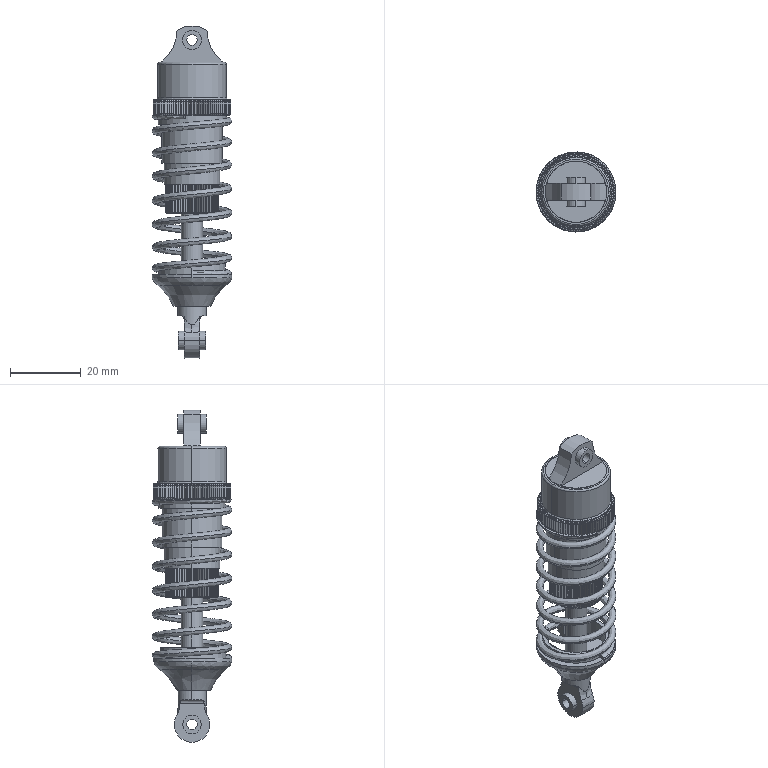Part | SolidWorks | features BaseBody 4 | 4 solids | 989 faces | box 22.605 x 22.6 x 94.05 mm | volume 15306 mm3 | cylinder 402 | plane 391 | spline 192 | torus 4 | commonest cylinder face diameters 1 x360 3 x4 5.2 x4 5.4 x4 17 x4 19 x4